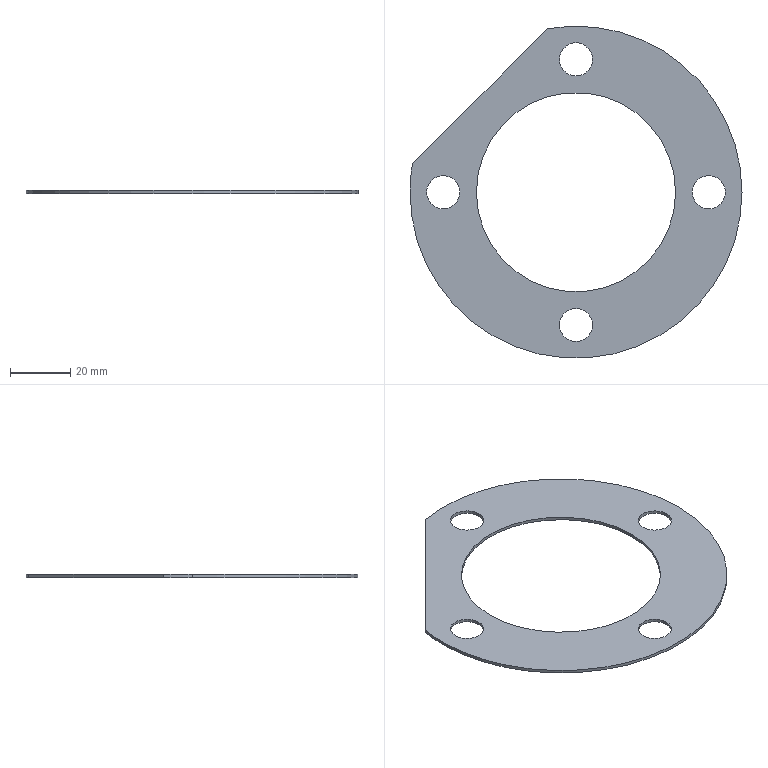Part | SolidWorks | features BaseBody 1 | 1 solid | 16 faces | box 110 x 110 x 1 mm | volume 5272 mm3 | cylinder 13 | plane 3 | commonest cylinder face diameters 11 x8 110 x3 66 x2
STEP:
#1=CARTESIAN_POINT('',(5.5,0.,0.));
#2=VERTEX_POINT('',#1);
#3=CARTESIAN_POINT('',(16.5,0.,0.));
#4=VERTEX_POINT('',#3);
#5=CARTESIAN_POINT('',(11.,0.,0.));
#6=DIRECTION('',(0.,0.,1.));
#7=DIRECTION('',(1.,0.,0.));
#8=AXIS2_PLACEMENT_3D('',#5,#6,#7);
#9=CIRCLE('',#8,5.5);
#10=EDGE_CURVE('',#2,#4,#9,.T.);
#11=ORIENTED_EDGE('',*,*,#10,.F.);
#12=CARTESIAN_POINT('',(5.5,0.,1.));
#13=VERTEX_POINT('',#12);
#14=CARTESIAN_POINT('',(5.5,0.,0.));
#15=DIRECTION('',(0.,0.,1.));
#16=VECTOR('',#15,1000.);
#17=LINE('',#14,#16);
#18=EDGE_CURVE('',#2,#13,#17,.T.);
#19=ORIENTED_EDGE('',*,*,#18,.T.);
#20=CARTESIAN_POINT('',(16.5,0.,1.));
#21=VERTEX_POINT('',#20);
#22=CARTESIAN_POINT('',(11.,0.,1.));
#23=DIRECTION('',(0.,0.,-1.));
#24=DIRECTION('',(1.,0.,0.));
#25=AXIS2_PLACEMENT_3D('',#22,#23,#24);
#26=CIRCLE('',#25,5.5);
#27=EDGE_CURVE('',#21,#13,#26,.T.);
#28=ORIENTED_EDGE('',*,*,#27,.F.);
#29=CARTESIAN_POINT('',(16.5,0.,0.));
#30=DIRECTION('',(0.,0.,1.));
#31=VECTOR('',#30,1000.);
#32=LINE('',#29,#31);
#33=EDGE_CURVE('',#4,#21,#32,.T.);
#34=ORIENTED_EDGE('',*,*,#33,.F.);
#35=EDGE_LOOP('',(#11,#19,#28,#34));
#36=FACE_OUTER_BOUND('',#35,.T.);
#37=CARTESIAN_POINT('',(11.,0.,0.));
#38=DIRECTION('',(0.,0.,1.));
#39=DIRECTION('',(1.,0.,0.));
#40=AXIS2_PLACEMENT_3D('',#37,#38,#39);
#41=CYLINDRICAL_SURFACE('',#40,5.5);
#42=ADVANCED_FACE('',(#36),#41,.F.);
#43=CARTESIAN_POINT('',(49.5,44.,0.));
#44=VERTEX_POINT('',#43);
#45=CARTESIAN_POINT('',(60.5,44.,0.));
#46=VERTEX_POINT('',#45);
#47=CARTESIAN_POINT('',(55.,44.,0.));
#48=DIRECTION('',(0.,0.,1.));
#49=DIRECTION('',(1.,0.,0.));
#50=AXIS2_PLACEMENT_3D('',#47,#48,#49);
#51=CIRCLE('',#50,5.5);
#52=EDGE_CURVE('',#44,#46,#51,.T.);
#53=ORIENTED_EDGE('',*,*,#52,.F.);
#54=CARTESIAN_POINT('',(49.5,44.,1.));
#55=VERTEX_POINT('',#54);
#56=CARTESIAN_POINT('',(49.5,44.,0.));
#57=DIRECTION('',(0.,0.,1.));
#58=VECTOR('',#57,1000.);
#59=LINE('',#56,#58);
#60=EDGE_CURVE('',#44,#55,#59,.T.);
#61=ORIENTED_EDGE('',*,*,#60,.T.);
#62=CARTESIAN_POINT('',(60.5,44.,1.));
#63=VERTEX_POINT('',#62);
#64=CARTESIAN_POINT('',(55.,44.,1.));
#65=DIRECTION('',(0.,0.,-1.));
#66=DIRECTION('',(1.,0.,0.));
#67=AXIS2_PLACEMENT_3D('',#64,#65,#66);
#68=CIRCLE('',#67,5.5);
#69=EDGE_CURVE('',#63,#55,#68,.T.);
#70=ORIENTED_EDGE('',*,*,#69,.F.);
#71=CARTESIAN_POINT('',(60.5,44.,0.));
#72=DIRECTION('',(0.,0.,1.));
#73=VECTOR('',#72,1000.);
#74=LINE('',#71,#73);
#75=EDGE_CURVE('',#46,#63,#74,.T.);
#76=ORIENTED_EDGE('',*,*,#75,.F.);
#77=EDGE_LOOP('',(#53,#61,#70,#76));
#78=FACE_OUTER_BOUND('',#77,.T.);
#79=CARTESIAN_POINT('',(55.,44.,0.));
#80=DIRECTION('',(0.,0.,1.));
#81=DIRECTION('',(1.,0.,0.));
#82=AXIS2_PLACEMENT_3D('',#79,#80,#81);
#83=CYLINDRICAL_SURFACE('',#82,5.5);
#84=ADVANCED_FACE('',(#78),#83,.F.);
#85=CARTESIAN_POINT('',(93.5,0.,0.));
#86=VERTEX_POINT('',#85);
#87=CARTESIAN_POINT('',(104.5,0.,0.));
#88=VERTEX_POINT('',#87);
#89=CARTESIAN_POINT('',(99.,0.,0.));
#90=DIRECTION('',(0.,0.,1.));
#91=DIRECTION('',(1.,0.,0.));
#92=AXIS2_PLACEMENT_3D('',#89,#90,#91);
#93=CIRCLE('',#92,5.5);
#94=EDGE_CURVE('',#86,#88,#93,.T.);
#95=ORIENTED_EDGE('',*,*,#94,.F.);
#96=CARTESIAN_POINT('',(93.5,0.,1.));
#97=VERTEX_POINT('',#96);
#98=CARTESIAN_POINT('',(93.5,0.,0.));
#99=DIRECTION('',(0.,0.,1.));
#100=VECTOR('',#99,1000.);
#101=LINE('',#98,#100);
#102=EDGE_CURVE('',#86,#97,#101,.T.);
#103=ORIENTED_EDGE('',*,*,#102,.T.);
#104=CARTESIAN_POINT('',(104.5,0.,1.));
#105=VERTEX_POINT('',#104);
#106=CARTESIAN_POINT('',(99.,0.,1.));
#107=DIRECTION('',(0.,0.,-1.));
#108=DIRECTION('',(1.,0.,0.));
#109=AXIS2_PLACEMENT_3D('',#106,#107,#108);
#110=CIRCLE('',#109,5.5);
#111=EDGE_CURVE('',#105,#97,#110,.T.);
#112=ORIENTED_EDGE('',*,*,#111,.F.);
#113=CARTESIAN_POINT('',(104.5,0.,0.));
#114=DIRECTION('',(0.,0.,1.));
#115=VECTOR('',#114,1000.);
#116=LINE('',#113,#115);
#117=EDGE_CURVE('',#88,#105,#116,.T.);
#118=ORIENTED_EDGE('',*,*,#117,.F.);
#119=EDGE_LOOP('',(#95,#103,#112,#118));
#120=FACE_OUTER_BOUND('',#119,.T.);
#121=CARTESIAN_POINT('',(99.,0.,0.));
#122=DIRECTION('',(0.,0.,1.));
#123=DIRECTION('',(1.,0.,0.));
#124=AXIS2_PLACEMENT_3D('',#121,#122,#123);
#125=CYLINDRICAL_SURFACE('',#124,5.5);
#126=ADVANCED_FACE('',(#120),#125,.F.);
#127=CARTESIAN_POINT('',(49.5,-44.,0.));
#128=VERTEX_POINT('',#127);
#129=CARTESIAN_POINT('',(60.5,-44.,0.));
#130=VERTEX_POINT('',#129);
#131=CARTESIAN_POINT('',(55.,-44.,0.));
#132=DIRECTION('',(0.,0.,1.));
#133=DIRECTION('',(1.,0.,0.));
#134=AXIS2_PLACEMENT_3D('',#131,#132,#133);
#135=CIRCLE('',#134,5.5);
#136=EDGE_CURVE('',#128,#130,#135,.T.);
#137=ORIENTED_EDGE('',*,*,#136,.F.);
#138=CARTESIAN_POINT('',(49.5,-44.,1.));
#139=VERTEX_POINT('',#138);
#140=CARTESIAN_POINT('',(49.5,-44.,0.));
#141=DIRECTION('',(0.,0.,1.));
#142=VECTOR('',#141,1000.);
#143=LINE('',#140,#142);
#144=EDGE_CURVE('',#128,#139,#143,.T.);
#145=ORIENTED_EDGE('',*,*,#144,.T.);
#146=CARTESIAN_POINT('',(60.5,-44.,1.));
#147=VERTEX_POINT('',#146);
#148=CARTESIAN_POINT('',(55.,-44.,1.));
#149=DIRECTION('',(0.,0.,-1.));
#150=DIRECTION('',(1.,0.,0.));
#151=AXIS2_PLACEMENT_3D('',#148,#149,#150);
#152=CIRCLE('',#151,5.5);
#153=EDGE_CURVE('',#147,#139,#152,.T.);
#154=ORIENTED_EDGE('',*,*,#153,.F.);
#155=CARTESIAN_POINT('',(60.5,-44.,0.));
#156=DIRECTION('',(0.,0.,1.));
#157=VECTOR('',#156,1000.);
#158=LINE('',#155,#157);
#159=EDGE_CURVE('',#130,#147,#158,.T.);
#160=ORIENTED_EDGE('',*,*,#159,.F.);
#161=EDGE_LOOP('',(#137,#145,#154,#160));
#162=FACE_OUTER_BOUND('',#161,.T.);
#163=CARTESIAN_POINT('',(55.,-44.,0.));
#164=DIRECTION('',(0.,0.,1.));
#165=DIRECTION('',(1.,0.,0.));
#166=AXIS2_PLACEMENT_3D('',#163,#164,#165);
#167=CYLINDRICAL_SURFACE('',#166,5.5);
#168=ADVANCED_FACE('',(#162),#167,.F.);
#169=CARTESIAN_POINT('',(22.,0.,0.));
#170=VERTEX_POINT('',#169);
#171=CARTESIAN_POINT('',(88.,0.,0.));
#172=VERTEX_POINT('',#171);
#173=CARTESIAN_POINT('',(55.,0.,0.));
#174=DIRECTION('',(0.,0.,1.));
#175=DIRECTION('',(1.,0.,0.));
#176=AXIS2_PLACEMENT_3D('',#173,#174,#175);
#177=CIRCLE('',#176,33.);
#178=EDGE_CURVE('',#170,#172,#177,.T.);
#179=ORIENTED_EDGE('',*,*,#178,.F.);
#180=CARTESIAN_POINT('',(22.,0.,1.));
#181=VERTEX_POINT('',#180);
#182=CARTESIAN_POINT('',(22.,0.,0.));
#183=DIRECTION('',(0.,0.,1.));
#184=VECTOR('',#183,1000.);
#185=LINE('',#182,#184);
#186=EDGE_CURVE('',#170,#181,#185,.T.);
#187=ORIENTED_EDGE('',*,*,#186,.T.);
#188=CARTESIAN_POINT('',(88.,0.,1.));
#189=VERTEX_POINT('',#188);
#190=CARTESIAN_POINT('',(55.,0.,1.));
#191=DIRECTION('',(0.,0.,-1.));
#192=DIRECTION('',(1.,0.,0.));
#193=AXIS2_PLACEMENT_3D('',#190,#191,#192);
#194=CIRCLE('',#193,33.);
#195=EDGE_CURVE('',#189,#181,#194,.T.);
#196=ORIENTED_EDGE('',*,*,#195,.F.);
#197=CARTESIAN_POINT('',(88.,0.,0.));
#198=DIRECTION('',(0.,0.,1.));
#199=VECTOR('',#198,1000.);
#200=LINE('',#197,#199);
#201=EDGE_CURVE('',#172,#189,#200,.T.);
#202=ORIENTED_EDGE('',*,*,#201,.F.);
#203=EDGE_LOOP('',(#179,#187,#196,#202));
#204=FACE_OUTER_BOUND('',#203,.T.);
#205=CARTESIAN_POINT('',(55.,0.,0.));
#206=DIRECTION('',(0.,0.,1.));
#207=DIRECTION('',(1.,0.,0.));
#208=AXIS2_PLACEMENT_3D('',#205,#206,#207);
#209=CYLINDRICAL_SURFACE('',#208,33.);
#210=ADVANCED_FACE('',(#204),#209,.F.);
#211=CARTESIAN_POINT('',(0.8195,9.459,0.));
#212=VERTEX_POINT('',#211);
#213=CARTESIAN_POINT('',(0.,0.,0.));
#214=VERTEX_POINT('',#213);
#215=CARTESIAN_POINT('',(55.,0.,0.));
#216=DIRECTION('',(0.,0.,1.));
#217=DIRECTION('',(1.,0.,0.));
#218=AXIS2_PLACEMENT_3D('',#215,#216,#217);
#219=CIRCLE('',#218,55.);
#220=EDGE_CURVE('',#212,#214,#219,.T.);
#221=ORIENTED_EDGE('',*,*,#220,.T.);
#222=CARTESIAN_POINT('',(0.,0.,1.));
#223=VERTEX_POINT('',#222);
#224=CARTESIAN_POINT('',(0.,0.,0.));
#225=DIRECTION('',(0.,0.,1.));
#226=VECTOR('',#225,1000.);
#227=LINE('',#224,#226);
#228=EDGE_CURVE('',#214,#223,#227,.T.);
#229=ORIENTED_EDGE('',*,*,#228,.T.);
#230=CARTESIAN_POINT('',(0.8195,9.459,1.));
#231=VERTEX_POINT('',#230);
#232=CARTESIAN_POINT('',(55.,0.,1.));
#233=DIRECTION('',(0.,0.,1.));
#234=DIRECTION('',(1.,0.,0.));
#235=AXIS2_PLACEMENT_3D('',#232,#233,#234);
#236=CIRCLE('',#235,55.);
#237=EDGE_CURVE('',#231,#223,#236,.T.);
#238=ORIENTED_EDGE('',*,*,#237,.F.);
#239=CARTESIAN_POINT('',(0.8195,9.459,0.));
#240=DIRECTION('',(0.,0.,-1.));
#241=VECTOR('',#240,1000.);
#242=LINE('',#239,#241);
#243=EDGE_CURVE('',#231,#212,#242,.T.);
#244=ORIENTED_EDGE('',*,*,#243,.T.);
#245=EDGE_LOOP('',(#221,#229,#238,#244));
#246=FACE_OUTER_BOUND('',#245,.T.);
#247=CARTESIAN_POINT('',(55.,0.,0.));
#248=DIRECTION('',(0.,0.,1.));
#249=DIRECTION('',(1.,0.,0.));
#250=AXIS2_PLACEMENT_3D('',#247,#248,#249);
#251=CYLINDRICAL_SURFACE('',#250,55.);
#252=ADVANCED_FACE('',(#246),#251,.T.);
#253=ORIENTED_EDGE('',*,*,#228,.F.);
#254=CARTESIAN_POINT('',(110.,0.,0.));
#255=VERTEX_POINT('',#254);
#256=CARTESIAN_POINT('',(55.,0.,0.));
#257=DIRECTION('',(0.,0.,1.));
#258=DIRECTION('',(1.,0.,0.));
#259=AXIS2_PLACEMENT_3D('',#256,#257,#258);
#260=CIRCLE('',#259,55.);
#261=EDGE_CURVE('',#214,#255,#260,.T.);
#262=ORIENTED_EDGE('',*,*,#261,.T.);
#263=CARTESIAN_POINT('',(110.,0.,1.));
#264=VERTEX_POINT('',#263);
#265=CARTESIAN_POINT('',(110.,0.,0.));
#266=DIRECTION('',(0.,0.,1.));
#267=VECTOR('',#266,1000.);
#268=LINE('',#265,#267);
#269=EDGE_CURVE('',#255,#264,#268,.T.);
#270=ORIENTED_EDGE('',*,*,#269,.T.);
#271=CARTESIAN_POINT('',(55.,0.,1.));
#272=DIRECTION('',(0.,0.,1.));
#273=DIRECTION('',(1.,0.,0.));
#274=AXIS2_PLACEMENT_3D('',#271,#272,#273);
#275=CIRCLE('',#274,55.);
#276=EDGE_CURVE('',#223,#264,#275,.T.);
#277=ORIENTED_EDGE('',*,*,#276,.F.);
#278=EDGE_LOOP('',(#253,#262,#270,#277));
#279=FACE_OUTER_BOUND('',#278,.T.);
#280=CARTESIAN_POINT('',(55.,0.,0.));
#281=DIRECTION('',(0.,0.,1.));
#282=DIRECTION('',(1.,0.,0.));
#283=AXIS2_PLACEMENT_3D('',#280,#281,#282);
#284=CYLINDRICAL_SURFACE('',#283,55.);
#285=ADVANCED_FACE('',(#279),#284,.T.);
#286=ORIENTED_EDGE('',*,*,#27,.T.);
#287=CARTESIAN_POINT('',(11.,0.,1.));
#288=DIRECTION('',(0.,0.,-1.));
#289=DIRECTION('',(1.,0.,0.));
#290=AXIS2_PLACEMENT_3D('',#287,#288,#289);
#291=CIRCLE('',#290,5.5);
#292=EDGE_CURVE('',#13,#21,#291,.T.);
#293=ORIENTED_EDGE('',*,*,#292,.T.);
#294=EDGE_LOOP('',(#286,#293));
#295=FACE_BOUND('',#294,.T.);
#296=ORIENTED_EDGE('',*,*,#69,.T.);
#297=CARTESIAN_POINT('',(55.,44.,1.));
#298=DIRECTION('',(0.,0.,-1.));
#299=DIRECTION('',(1.,0.,0.));
#300=AXIS2_PLACEMENT_3D('',#297,#298,#299);
#301=CIRCLE('',#300,5.5);
#302=EDGE_CURVE('',#55,#63,#301,.T.);
#303=ORIENTED_EDGE('',*,*,#302,.T.);
#304=EDGE_LOOP('',(#296,#303));
#305=FACE_BOUND('',#304,.T.);
#306=ORIENTED_EDGE('',*,*,#111,.T.);
#307=CARTESIAN_POINT('',(99.,0.,1.));
#308=DIRECTION('',(0.,0.,-1.));
#309=DIRECTION('',(1.,0.,0.));
#310=AXIS2_PLACEMENT_3D('',#307,#308,#309);
#311=CIRCLE('',#310,5.5);
#312=EDGE_CURVE('',#97,#105,#311,.T.);
#313=ORIENTED_EDGE('',*,*,#312,.T.);
#314=EDGE_LOOP('',(#306,#313));
#315=FACE_BOUND('',#314,.T.);
#316=ORIENTED_EDGE('',*,*,#153,.T.);
#317=CARTESIAN_POINT('',(55.,-44.,1.));
#318=DIRECTION('',(0.,0.,-1.));
#319=DIRECTION('',(1.,0.,0.));
#320=AXIS2_PLACEMENT_3D('',#317,#318,#319);
#321=CIRCLE('',#320,5.5);
#322=EDGE_CURVE('',#139,#147,#321,.T.);
#323=ORIENTED_EDGE('',*,*,#322,.T.);
#324=EDGE_LOOP('',(#316,#323));
#325=FACE_BOUND('',#324,.T.);
#326=ORIENTED_EDGE('',*,*,#195,.T.);
#327=CARTESIAN_POINT('',(55.,0.,1.));
#328=DIRECTION('',(0.,0.,-1.));
#329=DIRECTION('',(1.,0.,0.));
#330=AXIS2_PLACEMENT_3D('',#327,#328,#329);
#331=CIRCLE('',#330,33.);
#332=EDGE_CURVE('',#181,#189,#331,.T.);
#333=ORIENTED_EDGE('',*,*,#332,.T.);
#334=EDGE_LOOP('',(#326,#333));
#335=FACE_BOUND('',#334,.T.);
#336=CARTESIAN_POINT('',(45.541,54.18,1.));
#337=VERTEX_POINT('',#336);
#338=CARTESIAN_POINT('',(45.541,54.18,1.));
#339=DIRECTION('',(-0.7071,-0.7071,0.));
#340=VECTOR('',#339,1000.);
#341=LINE('',#338,#340);
#342=EDGE_CURVE('',#337,#231,#341,.T.);
#343=ORIENTED_EDGE('',*,*,#342,.T.);
#344=ORIENTED_EDGE('',*,*,#237,.T.);
#345=ORIENTED_EDGE('',*,*,#276,.T.);
#346=CARTESIAN_POINT('',(55.,0.,1.));
#347=DIRECTION('',(0.,0.,1.));
#348=DIRECTION('',(1.,0.,0.));
#349=AXIS2_PLACEMENT_3D('',#346,#347,#348);
#350=CIRCLE('',#349,55.);
#351=EDGE_CURVE('',#264,#337,#350,.T.);
#352=ORIENTED_EDGE('',*,*,#351,.T.);
#353=EDGE_LOOP('',(#343,#344,#345,#352));
#354=FACE_OUTER_BOUND('',#353,.T.);
#355=CARTESIAN_POINT('',(54.383,0.6168,1.));
#356=DIRECTION('',(0.,0.,1.));
#357=DIRECTION('',(1.,0.,0.));
#358=AXIS2_PLACEMENT_3D('',#355,#356,#357);
#359=PLANE('',#358);
#360=ADVANCED_FACE('',(#295,#305,#315,#325,#335,#354),#359,.T.);
#361=ORIENTED_EDGE('',*,*,#18,.F.);
#362=CARTESIAN_POINT('',(11.,0.,0.));
#363=DIRECTION('',(0.,0.,1.));
#364=DIRECTION('',(1.,0.,0.));
#365=AXIS2_PLACEMENT_3D('',#362,#363,#364);
#366=CIRCLE('',#365,5.5);
#367=EDGE_CURVE('',#4,#2,#366,.T.);
#368=ORIENTED_EDGE('',*,*,#367,.F.);
#369=ORIENTED_EDGE('',*,*,#33,.T.);
#370=ORIENTED_EDGE('',*,*,#292,.F.);
#371=EDGE_LOOP('',(#361,#368,#369,#370));
#372=FACE_OUTER_BOUND('',#371,.T.);
#373=CARTESIAN_POINT('',(11.,0.,0.));
#374=DIRECTION('',(0.,0.,1.));
#375=DIRECTION('',(1.,0.,0.));
#376=AXIS2_PLACEMENT_3D('',#373,#374,#375);
#377=CYLINDRICAL_SURFACE('',#376,5.5);
#378=ADVANCED_FACE('',(#372),#377,.F.);
#379=ORIENTED_EDGE('',*,*,#60,.F.);
#380=CARTESIAN_POINT('',(55.,44.,0.));
#381=DIRECTION('',(0.,0.,1.));
#382=DIRECTION('',(1.,0.,0.));
#383=AXIS2_PLACEMENT_3D('',#380,#381,#382);
#384=CIRCLE('',#383,5.5);
#385=EDGE_CURVE('',#46,#44,#384,.T.);
#386=ORIENTED_EDGE('',*,*,#385,.F.);
#387=ORIENTED_EDGE('',*,*,#75,.T.);
#388=ORIENTED_EDGE('',*,*,#302,.F.);
#389=EDGE_LOOP('',(#379,#386,#387,#388));
#390=FACE_OUTER_BOUND('',#389,.T.);
#391=CARTESIAN_POINT('',(55.,44.,0.));
#392=DIRECTION('',(0.,0.,1.));
#393=DIRECTION('',(1.,0.,0.));
#394=AXIS2_PLACEMENT_3D('',#391,#392,#393);
#395=CYLINDRICAL_SURFACE('',#394,5.5);
#396=ADVANCED_FACE('',(#390),#395,.F.);
#397=ORIENTED_EDGE('',*,*,#102,.F.);
#398=CARTESIAN_POINT('',(99.,0.,0.));
#399=DIRECTION('',(0.,0.,1.));
#400=DIRECTION('',(1.,0.,0.));
#401=AXIS2_PLACEMENT_3D('',#398,#399,#400);
#402=CIRCLE('',#401,5.5);
#403=EDGE_CURVE('',#88,#86,#402,.T.);
#404=ORIENTED_EDGE('',*,*,#403,.F.);
#405=ORIENTED_EDGE('',*,*,#117,.T.);
#406=ORIENTED_EDGE('',*,*,#312,.F.);
#407=EDGE_LOOP('',(#397,#404,#405,#406));
#408=FACE_OUTER_BOUND('',#407,.T.);
#409=CARTESIAN_POINT('',(99.,0.,0.));
#410=DIRECTION('',(0.,0.,1.));
#411=DIRECTION('',(1.,0.,0.));
#412=AXIS2_PLACEMENT_3D('',#409,#410,#411);
#413=CYLINDRICAL_SURFACE('',#412,5.5);
#414=ADVANCED_FACE('',(#408),#413,.F.);
#415=ORIENTED_EDGE('',*,*,#144,.F.);
#416=CARTESIAN_POINT('',(55.,-44.,0.));
#417=DIRECTION('',(0.,0.,1.));
#418=DIRECTION('',(1.,0.,0.));
#419=AXIS2_PLACEMENT_3D('',#416,#417,#418);
#420=CIRCLE('',#419,5.5);
#421=EDGE_CURVE('',#130,#128,#420,.T.);
#422=ORIENTED_EDGE('',*,*,#421,.F.);
#423=ORIENTED_EDGE('',*,*,#159,.T.);
#424=ORIENTED_EDGE('',*,*,#322,.F.);
#425=EDGE_LOOP('',(#415,#422,#423,#424));
#426=FACE_OUTER_BOUND('',#425,.T.);
#427=CARTESIAN_POINT('',(55.,-44.,0.));
#428=DIRECTION('',(0.,0.,1.));
#429=DIRECTION('',(1.,0.,0.));
#430=AXIS2_PLACEMENT_3D('',#427,#428,#429);
#431=CYLINDRICAL_SURFACE('',#430,5.5);
#432=ADVANCED_FACE('',(#426),#431,.F.);
#433=ORIENTED_EDGE('',*,*,#186,.F.);
#434=CARTESIAN_POINT('',(55.,0.,0.));
#435=DIRECTION('',(0.,0.,1.));
#436=DIRECTION('',(1.,0.,0.));
#437=AXIS2_PLACEMENT_3D('',#434,#435,#436);
#438=CIRCLE('',#437,33.);
#439=EDGE_CURVE('',#172,#170,#438,.T.);
#440=ORIENTED_EDGE('',*,*,#439,.F.);
#441=ORIENTED_EDGE('',*,*,#201,.T.);
#442=ORIENTED_EDGE('',*,*,#332,.F.);
#443=EDGE_LOOP('',(#433,#440,#441,#442));
#444=FACE_OUTER_BOUND('',#443,.T.);
#445=CARTESIAN_POINT('',(55.,0.,0.));
#446=DIRECTION('',(0.,0.,1.));
#447=DIRECTION('',(1.,0.,0.));
#448=AXIS2_PLACEMENT_3D('',#445,#446,#447);
#449=CYLINDRICAL_SURFACE('',#448,33.);
#450=ADVANCED_FACE('',(#444),#449,.F.);
#451=ORIENTED_EDGE('',*,*,#269,.F.);
#452=CARTESIAN_POINT('',(45.541,54.18,0.));
#453=VERTEX_POINT('',#452);
#454=CARTESIAN_POINT('',(55.,0.,0.));
#455=DIRECTION('',(0.,0.,1.));
#456=DIRECTION('',(1.,0.,0.));
#457=AXIS2_PLACEMENT_3D('',#454,#455,#456);
#458=CIRCLE('',#457,55.);
#459=EDGE_CURVE('',#255,#453,#458,.T.);
#460=ORIENTED_EDGE('',*,*,#459,.T.);
#461=CARTESIAN_POINT('',(45.541,54.18,0.));
#462=DIRECTION('',(0.,0.,1.));
#463=VECTOR('',#462,1000.);
#464=LINE('',#461,#463);
#465=EDGE_CURVE('',#453,#337,#464,.T.);
#466=ORIENTED_EDGE('',*,*,#465,.T.);
#467=ORIENTED_EDGE('',*,*,#351,.F.);
#468=EDGE_LOOP('',(#451,#460,#466,#467));
#469=FACE_OUTER_BOUND('',#468,.T.);
#470=CARTESIAN_POINT('',(55.,0.,0.));
#471=DIRECTION('',(0.,0.,1.));
#472=DIRECTION('',(1.,0.,0.));
#473=AXIS2_PLACEMENT_3D('',#470,#471,#472);
#474=CYLINDRICAL_SURFACE('',#473,55.);
#475=ADVANCED_FACE('',(#469),#474,.T.);
#476=ORIENTED_EDGE('',*,*,#342,.F.);
#477=ORIENTED_EDGE('',*,*,#465,.F.);
#478=CARTESIAN_POINT('',(45.541,54.18,0.));
#479=DIRECTION('',(-0.7071,-0.7071,0.));
#480=VECTOR('',#479,1000.);
#481=LINE('',#478,#480);
#482=EDGE_CURVE('',#453,#212,#481,.T.);
#483=ORIENTED_EDGE('',*,*,#482,.T.);
#484=ORIENTED_EDGE('',*,*,#243,.F.);
#485=EDGE_LOOP('',(#476,#477,#483,#484));
#486=FACE_OUTER_BOUND('',#485,.T.);
#487=CARTESIAN_POINT('',(45.541,54.18,0.));
#488=DIRECTION('',(-0.7071,0.7071,0.));
#489=DIRECTION('',(-0.7071,-0.7071,0.));
#490=AXIS2_PLACEMENT_3D('',#487,#488,#489);
#491=PLANE('',#490);
#492=ADVANCED_FACE('',(#486),#491,.T.);
#493=ORIENTED_EDGE('',*,*,#367,.T.);
#494=ORIENTED_EDGE('',*,*,#10,.T.);
#495=EDGE_LOOP('',(#493,#494));
#496=FACE_BOUND('',#495,.T.);
#497=ORIENTED_EDGE('',*,*,#385,.T.);
#498=ORIENTED_EDGE('',*,*,#52,.T.);
#499=EDGE_LOOP('',(#497,#498));
#500=FACE_BOUND('',#499,.T.);
#501=ORIENTED_EDGE('',*,*,#403,.T.);
#502=ORIENTED_EDGE('',*,*,#94,.T.);
#503=EDGE_LOOP('',(#501,#502));
#504=FACE_BOUND('',#503,.T.);
#505=ORIENTED_EDGE('',*,*,#421,.T.);
#506=ORIENTED_EDGE('',*,*,#136,.T.);
#507=EDGE_LOOP('',(#505,#506));
#508=FACE_BOUND('',#507,.T.);
#509=ORIENTED_EDGE('',*,*,#439,.T.);
#510=ORIENTED_EDGE('',*,*,#178,.T.);
#511=EDGE_LOOP('',(#509,#510));
#512=FACE_BOUND('',#511,.T.);
#513=ORIENTED_EDGE('',*,*,#220,.F.);
#514=ORIENTED_EDGE('',*,*,#482,.F.);
#515=ORIENTED_EDGE('',*,*,#459,.F.);
#516=ORIENTED_EDGE('',*,*,#261,.F.);
#517=EDGE_LOOP('',(#513,#514,#515,#516));
#518=FACE_OUTER_BOUND('',#517,.T.);
#519=CARTESIAN_POINT('',(54.383,0.6168,0.));
#520=DIRECTION('',(0.,0.,1.));
#521=DIRECTION('',(1.,0.,0.));
#522=AXIS2_PLACEMENT_3D('',#519,#520,#521);
#523=PLANE('',#522);
#524=ADVANCED_FACE('',(#496,#500,#504,#508,#512,#518),#523,.F.);
#525=CLOSED_SHELL('',(#42,#84,#126,#168,#210,#252,#285,#360,#378,#396,#414,#432,#450,#475,#492,#524));
#526=MANIFOLD_SOLID_BREP('',#525);
#527=CARTESIAN_POINT('',(0.,0.,0.));
#528=DIRECTION('',(0.,0.,1.));
#529=DIRECTION('',(1.,0.,0.));
#530=AXIS2_PLACEMENT_3D('',#527,#528,#529);
#531=(LENGTH_UNIT()NAMED_UNIT(*)SI_UNIT(.MILLI.,.METRE.));
#532=UNCERTAINTY_MEASURE_WITH_UNIT(LENGTH_MEASURE(0.00001),#531,'','');
#533=(NAMED_UNIT(*)PLANE_ANGLE_UNIT()SI_UNIT($,.RADIAN.));
#534=(NAMED_UNIT(*)SI_UNIT($,.STERADIAN.)SOLID_ANGLE_UNIT());
#535=(GEOMETRIC_REPRESENTATION_CONTEXT(3)GLOBAL_UNCERTAINTY_ASSIGNED_CONTEXT((#532))GLOBAL_UNIT_ASSIGNED_CONTEXT((#531,#533,#534))REPRESENTATION_CONTEXT('',''));
#536=ADVANCED_BREP_SHAPE_REPRESENTATION('',(#526,#530),#535);